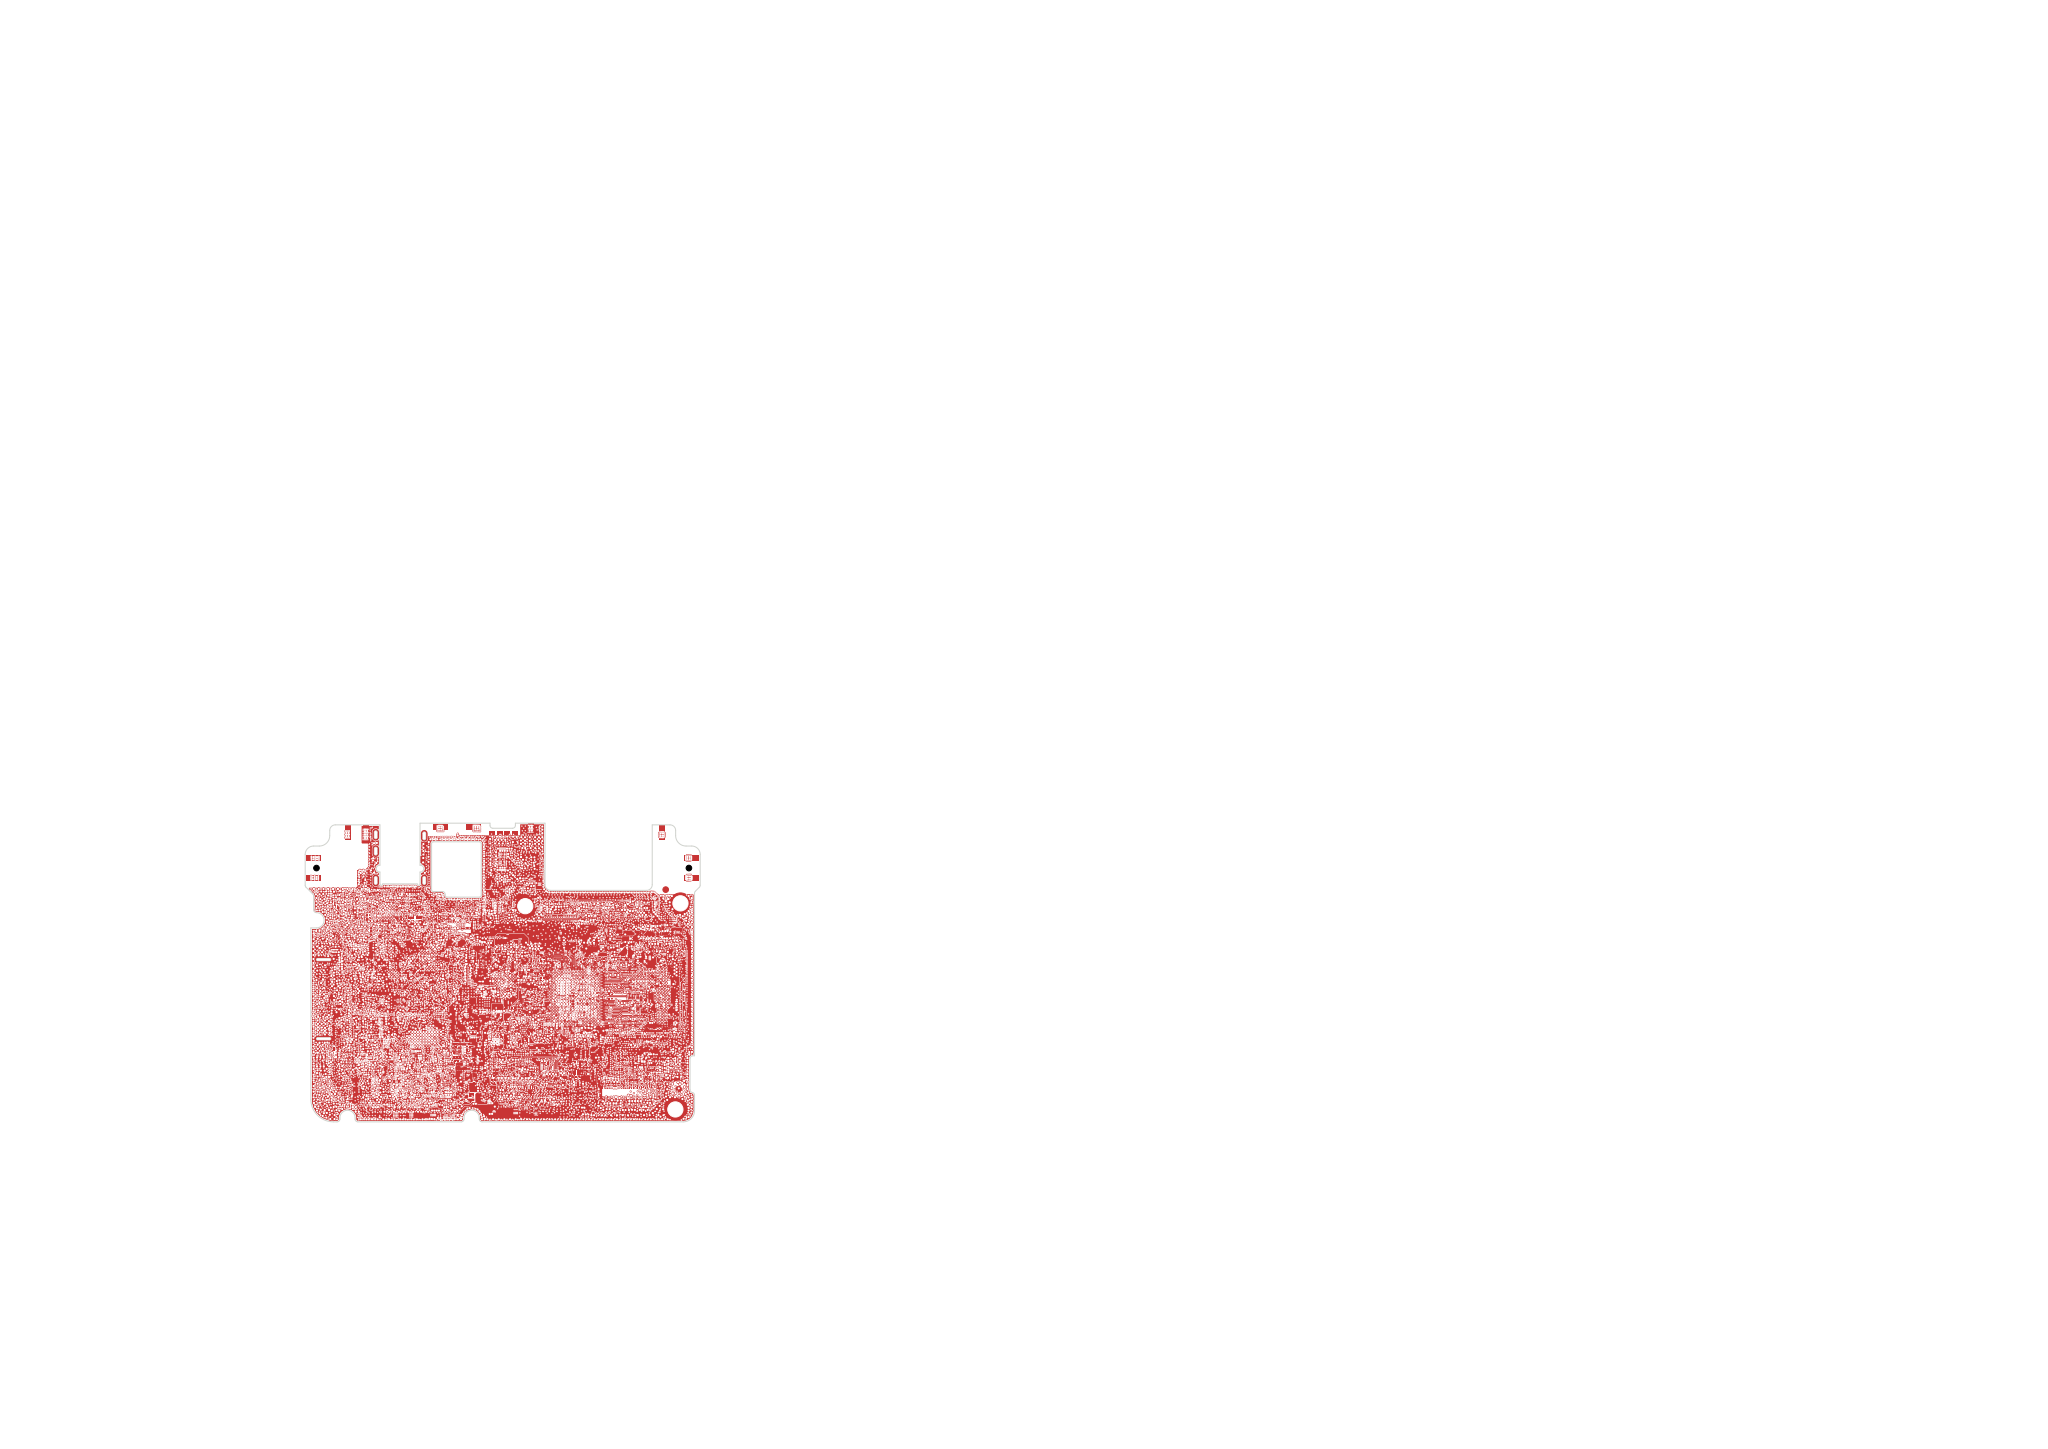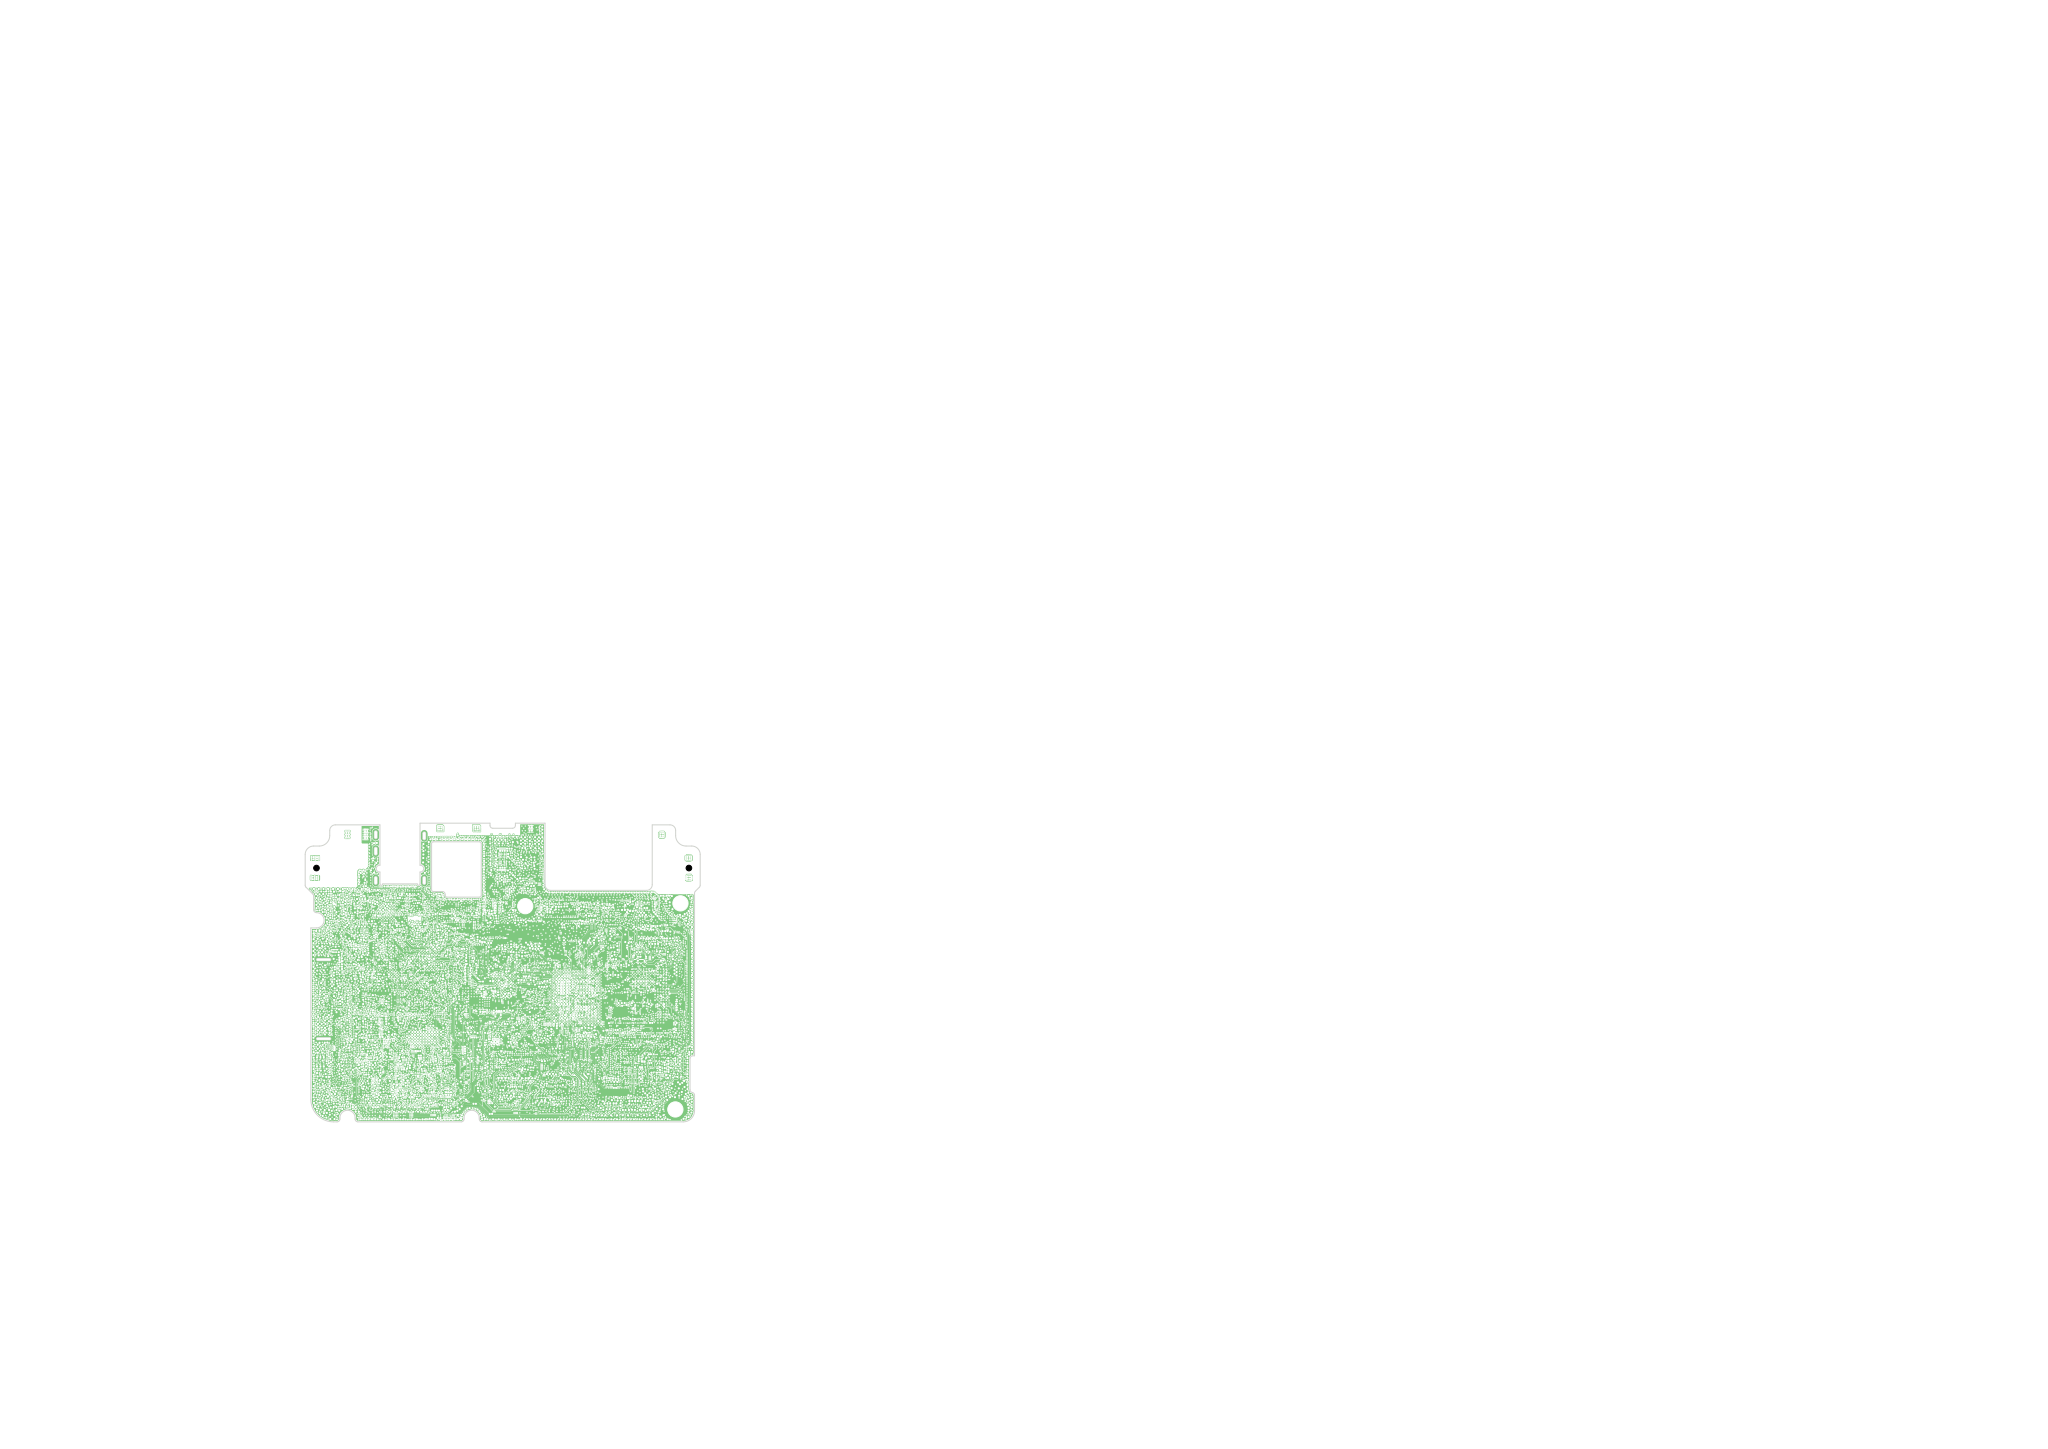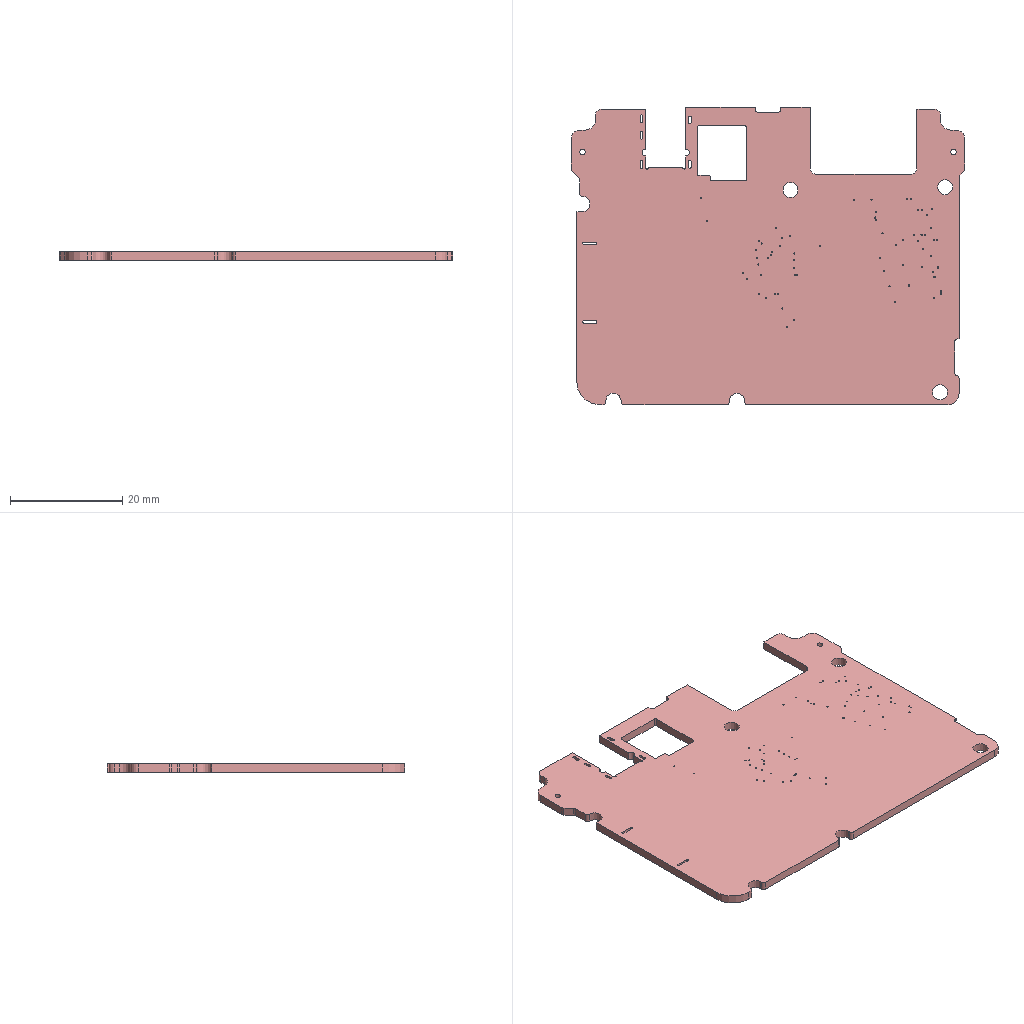Circuit board layout | KiCad | box 70 x 52.9 x 1.5 mm
Layer stack:
layer,type,thickness_mm,material,epsilon_r
F.Cu,copper (signal),,,
In1.Cu,copper (signal),,,
In2.Cu,copper (signal),,,
In3.Cu,copper (signal),,,
In4.Cu,copper (signal),,,
In5.Cu,copper (signal),,,
In6.Cu,copper (signal),,,
In7.Cu,copper (signal),,,
In8.Cu,copper (signal),,,
B.Cu,copper (signal),,,
# board thickness,1.6,,,
Part placement, first 811 of 1662 lines:
Ref,Val,Package,PosX,PosY,Rot,Side
B2102,,,26.012,28.75,-90,bottom
B2705,,,-11.025,38.45,180,bottom
C1101,,,9.938,26.938,-90,bottom
C1102,,,8.838,26.938,-90,bottom
C1103,,,12.137,24.312,0,bottom
C1104,,,12.137,23.712,0,bottom
C1105,,,11.387,26.3,-90,bottom
C1106,,,11.988,26.3,-90,bottom
C1107,,,12.137,24.913,0,bottom
C1108,,,12.588,25.988,-90,bottom
C1109,,,10.787,26.3,-90,bottom
C1111,,,9.338,19.5,180,bottom
C1122,,,8.2,21.7,0,bottom
C1123,,,9.338,18.4,180,bottom
C1124,,,8.2,20.6,0,bottom
C1125,,,9.938,23.712,0,bottom
C1126,,,9.938,23.113,0,bottom
C1127,,,9.938,22.512,0,bottom
C1128,,,11.037,24.913,180,bottom
C1129,,,11.037,23.712,180,bottom
C1130,,,11.037,23.113,180,bottom
C1131,,,6.237,17.288,0,bottom
C1132,,,8.537,17.288,180,bottom
C1133,,,11.6,20.712,180,bottom
C1134,,,9.938,24.913,0,bottom
C1135,,,11.037,19.95,180,bottom
C1136,,,10.5,21.312,0,bottom
C1137,,,10.5,20.712,0,bottom
C1138,,,11.6,21.312,180,bottom
C1139,,,11.037,24.312,180,bottom
C1140,,,11.037,22.512,180,bottom
C1170,,,9.938,24.312,0,bottom
C1171,,,14.463,29.062,0,bottom
C1172,,,14.463,30.163,0,bottom
C1173,,,12.387,22.863,90,bottom
C1174,,,15.8,25.137,0,bottom
C1175,,,14.7,25.137,180,bottom
C1176,,,13.225,23.15,-90,bottom
C1177,,,14.238,22.438,180,bottom
C1182,,,11.037,19.35,0,bottom
C1183,,,9.088,22.8,-90,bottom
C1201,,,11.04,18.75,180,bottom
C1202,,,15.537,20.212,0,bottom
C1203,,,13.225,24.25,90,bottom
C1204,,,9.65,20.962,90,bottom
C1205,,,13.338,19.2,0,bottom
C1211,,,18.2,22.562,-90,bottom
C1212,,,13.338,18.6,0,bottom
C1213,,,13.225,25.35,90,bottom
C1214,,,18.337,19.863,180,bottom
C1221,,,12.137,19.35,180,bottom
C1222,,,9.938,25.512,180,bottom
C1223,,,13.225,27.55,-90,bottom
C1224,,,13.225,26.45,90,bottom
C1225,,,15.537,18.413,0,bottom
C1231,,,11.037,18.15,180,bottom
C1232,,,11.6,21.913,0,bottom
C1241,,,10.588,17.3,90,bottom
C1242,,,17.038,17.562,180,bottom
C1243,,,15.537,19.012,180,bottom
C1244,,,14.438,19.012,0,bottom
C1245,,,14.438,18.413,0,bottom
C1246,,,14.438,20.4,180,bottom
C1247,,,14.438,19.8,180,bottom
C1248,,,15.537,19.613,180,bottom
C1249,,,14.338,17.562,0,bottom
C1251,,,15.55,25.988,-90,bottom
C1252,,,16.637,19.262,90,bottom
C1253,,,16.25,21.688,-90,bottom
C1254,,,18.337,18.762,180,bottom
C1255,,,15.15,23.938,180,bottom
C1256,,,15.15,23.337,180,bottom
C1257,,,13.338,19.913,0,bottom
C1258,,,13.338,20.512,0,bottom
C1259,,,13.338,21.113,0,bottom
C1260,,,14.488,21.587,-90,bottom
C1262,,,9.988,17.288,90,bottom
C1263,,,7.6,19.75,0,bottom
C1271,,,12.137,19.95,0,bottom
C1272,,,15.8,24.538,0,bottom
C1280,,,12.137,18.15,180,bottom
C1281,,,17.863,27.863,0,bottom
C1282,,,17.863,26.762,0,bottom
C1283,,,17.35,23.712,180,bottom
C1284,,,17.35,23.113,180,bottom
C1285,,,16.25,23.738,0,bottom
C1286,,,16.25,23.137,0,bottom
C1287,,,17.35,22.512,180,bottom
C1288,,,12.137,18.75,180,bottom
C1291,,,14.95,25.988,-90,bottom
C1501,,,2.15,28,-90,bottom
C1503,,,3.4,18.35,180,bottom
C1504,,,-2.05,27.7,180,bottom
C1507,,,0.1,29.65,180,bottom
C1508,,,1.025,20.2,0,bottom
C1509,,,-0.9375,18.637,0,bottom
C1519,,,1.587,18.337,180,bottom
C1525,,,2.45,30.3,-90,bottom
C1526,,,-0.25,31.1,-90,bottom
C1527,,,3.4,17.25,180,bottom
C1528,,,-1.85,28.5,180,bottom
C1529,,,-5.425,30.525,90,bottom
C1601,,,4.2,23.2,0,bottom
C1602,,,4.2,22.6,0,bottom
C1603,,,1.65,20.7,-90,bottom
C1604,,,4.05,26.95,0,bottom
C1605,,,3.9,30.3,0,bottom
C1606,,,3.9,31.4,0,bottom
C1607,,,4.188,25.125,0,bottom
C1612,,,4.812,25.875,0,bottom
C1613,,,-1.875,19.3,0,bottom
C1614,,,4.612,21.85,0,bottom
C1615,,,4.188,24.525,0,bottom
C1621,,,9.113,29.288,90,bottom
C1622,,,8.012,29.288,90,bottom
C1701,,,1.1,31.15,90,bottom
C1702,,,-4.1,27.25,180,bottom
C1703,,,0.95,27.95,90,bottom
C1704,,,-0.05,27.95,90,bottom
C1705,,,-1.55,29.5,90,bottom
C1706,,,-0.75,28.4,90,bottom
C1707,,,1.85,30.3,90,bottom
C1708,,,-3.9,25.85,180,bottom
C1709,,,-5.9,23,0,bottom
C1710,,,-4.1,28.05,180,bottom
C1711,,,11.162,29.988,90,bottom
C1712,,,1.05,29.55,90,bottom
C1713,,,0.1,30.25,180,bottom
C1714,,,-2.15,29.5,90,bottom
C1715,,,-0.95,29.5,90,bottom
C1716,,,-6.15,24,90,bottom
C1717,,,-5.15,26.45,180,bottom
C1718,,,-4.3,25,180,bottom
C1719,,,-3.9,26.55,0,bottom
C1720,,,-5.15,25.85,0,bottom
C1721,,,0.1,29.05,0,bottom
C1801,,,-4.15,24.125,90,bottom
C1802,,,-3.25,23.025,90,bottom
C1803,,,-1.09,20.575,-90,bottom
C1804,,,0.75,21.15,0,bottom
C1805,,,-4.9,23.85,90,bottom
C1807,,,-5.5,23.85,90,bottom
C1808,,,-0.75,19.35,180,bottom
C1809,,,-3.85,19.337,0,bottom
C1810,,,-1.475,16.837,180,bottom
C1811,,,-2.575,16.837,180,bottom
C1812,,,-3.4,23.9,90,bottom
C1828,,,-2.675,17.538,180,bottom
C1829,,,-5.1,22.15,180,bottom
C1834,,,-3.85,18.163,90,bottom
C1835,,,-4.525,17.175,90,bottom
C1901,,,24.5,21.85,-90,bottom
C1902,,,26.6,20.8,180,bottom
C1903,,,26.6,21.9,180,bottom
C1904,,,23.413,30,-90,bottom
C1905,,,23.212,17.3,90,bottom
C1906,,,23.1,18.663,-90,bottom
C1907,,,23.7,21.85,-90,bottom
C2001,,,22.2,22.1,-90,bottom
C2002,,,23.775,28.462,90,bottom
C2003,,,20.875,24.587,180,bottom
C2004,,,20.812,25.712,180,bottom
C2005,,,22.188,20.375,-90,bottom
C2006,,,20.7,29.65,90,bottom
C2007,,,19.413,26.812,90,bottom
C2008,,,19.812,28.012,180,bottom
C2009,,,22.538,19.525,0,bottom
C2010,,,30.375,20.775,0,bottom
C2011,,,28.175,21.275,-90,bottom
C2012,,,20.625,26.413,180,bottom
C2013,,,22.25,28.35,0,bottom
C2014,,,25.163,28.925,90,bottom
C2015,,,20.025,21.562,180,bottom
C2016,,,20.15,27.262,180,bottom
C2019,,,22.9,21.85,-90,bottom
C2020,,,22.788,20.375,-90,bottom
C2021,,,20.825,17.562,90,bottom
C2108,,,24.012,30,-90,bottom
C2109,,,24.613,30,90,bottom
C2110,,,25.212,30,90,bottom
C2111,,,28.01,28.348,0,bottom
C2118,,,26.812,28.75,-90,bottom
C2119,,,26.663,29.85,180,bottom
C2122,,,30.25,29.85,90,bottom
C2123,,,28.77,26.34,180,bottom
C2128,,,27.703,29.55,-90,bottom
C2129,,,25.812,30.1,90,bottom
C2130,,,28.378,30.65,180,bottom
C2131,,,26.075,31.25,180,bottom
C2132,,,26.075,31.85,180,bottom
C2133,,,26.925,31.6,90,bottom
C2134,,,28.375,31.85,180,bottom
C2135,,,27.525,31.6,90,bottom
C2201,,,28.45,22.125,180,bottom
C2202,,,29.05,22.875,0,bottom
C2203,,,28.2,23.775,180,bottom
C2204,,,31.3,25.25,-90,bottom
C2205,,,31.145,18.175,0,bottom
C2206,,,29.65,19.075,0,bottom
C2207,,,28.773,29.75,180,bottom
C2208,,,31.625,20.85,90,bottom
C2209,,,31.145,19.075,0,bottom
C2210,,,29.65,18.175,0,bottom
C2211,,,29,24.95,180,bottom
C2212,,,28.77,26.94,180,bottom
C2213,,,30.45,24.7,90,bottom
C2277,,,29.025,20.675,-90,bottom
C2707,,,-5.925,38.1,180,bottom
C2708,,,-12.475,38.45,-90,bottom
C2709,,,-6.675,37.5,0,bottom
C2710,,,-7.025,38.1,0,bottom
C2712,,,-9.325,37,180,bottom
C2718,,,2.875,41.95,90,bottom
C2730,,,6.25,42.8,180,bottom
C2731,,,4.225,42.8,0,bottom
C2732,,,5.025,40.6,0,bottom
C2755,,,-6.675,36.9,0,bottom
C3237,,,10.463,35.4,-90,bottom
C3238,,,9.863,35.4,-90,bottom
C3239,,,9.262,35.388,90,bottom
C3242,,,13.363,35.4,-90,bottom
C3243,,,9.662,39.612,90,bottom
C3244,,,14.887,39.625,-90,bottom
C3245,,,13.45,39.6,-90,bottom
C3246,,,14.05,39.6,-90,bottom
C3247,,,20.337,35.4,-90,bottom
C3248,,,19.738,35.4,-90,bottom
C3249,,,19.137,35.4,90,bottom
C3252,,,23.788,35.65,0,bottom
C3253,,,19.512,39.612,90,bottom
C3254,,,24.725,39.612,-90,bottom
C3255,,,24.125,39.612,-90,bottom
C3256,,,23.525,39.612,-90,bottom
C3351,,,0.7125,37.35,0,bottom
C3352,,,0,38.3,-90,bottom
C3702,,,11.588,14.8,0,bottom
C3713,,,6.388,14.2,180,bottom
C3717,,,14.599,9.125,90,bottom
C3718,,,10.75,10.05,90,bottom
C3719,,,9.55,10.05,90,bottom
C3800,,,-10.45,21.2,0,bottom
C3900,,,-15.975,25.85,-90,bottom
C3901,,,-16.15,28.75,0,bottom
C3902,,,-11.62,33.43,-90,bottom
C3903,,,-16.15,28.15,0,bottom
C3904,,,-11.7,34.675,0,bottom
C3905,,,-17.225,27.55,180,bottom
C3906,,,-10.375,34.3,90,bottom
C3907,,,-17,28.4,90,bottom
C3908,,,-10.97,34.3,90,bottom
C3909,,,-12,23.875,180,bottom
C3910,,,-15.125,25.575,180,bottom
C3911,,,-12.27,33.625,-90,bottom
C3912,,,-12.025,32.775,180,bottom
C3913,,,-12.85,23.975,90,bottom
C3914,,,-9.125,27.062,-90,bottom
C3915,,,-9.113,25.06,90,bottom
C3916,,,-9.75,29.82,-90,bottom
C3917,,,-9.515,34.935,180,bottom
C3918,,,-10,31.025,0,bottom
C3919,,,-9.1,30.975,90,bottom
C3920,,,-9.72,33.625,180,bottom
C3921,,,-10.885,33.195,90,bottom
C4001,,,-18.7,31.15,0,bottom
C4002,,,-10.5,32.075,-90,bottom
C4003,,,-19.8,31.15,0,bottom
C4004,,,-10.15,25.2,90,bottom
C4006,,,-18.6,30.55,0,bottom
C4007,,,-19.7,30.55,0,bottom
C4010,,,-19.7,29.95,0,bottom
C4011,,,-18.6,29.35,0,bottom
C4014,,,-17.275,34.15,180,bottom
C4015,,,-18.7,33.538,0,bottom
C4019,,,-18.6,29.95,0,bottom
C4020,,,-18.2,28.475,90,bottom
C4021,,,-18.7,32.95,0,bottom
C4022,,,-19.8,32.95,0,bottom
C4024,,,-19.8,32.35,0,bottom
C4026,,,-17.6,32.35,0,bottom
C4028,,,-19.8,31.75,0,bottom
C4029,,,-17.6,31.75,0,bottom
C4031,,,-15.425,33.175,-90,bottom
C4034,,,-14.825,33.175,-90,bottom
C4043,,,-14.225,33.775,-90,bottom
C4045,,,-15.075,34,0,bottom
C4046,,,-13.625,33.775,-90,bottom
C4047,,,-14.225,34.875,-90,bottom
C4048,,,-13.025,33.775,-90,bottom
C4049,,,-13.025,34.875,-90,bottom
C4050,,,-16.212,17.887,90,bottom
C4059,,,-15,17.887,90,bottom
C4062,,,-11.387,25.038,0,bottom
C4070,,,-17.6,17.887,90,bottom
C4071,,,-9.65,32.237,180,bottom
C4072,,,-12,24.475,0,bottom
C4073,,,-10.035,32.945,180,bottom
C4101,,,-12.75,11.725,0,bottom
C4102,,,-9.5,11.95,180,bottom
C4103,,,-18.575,15.675,0,bottom
C4104,,,-17.725,15.325,90,bottom
C4105,,,-12.562,17.887,-90,bottom
C4106,,,-11.463,17.738,180,bottom
C4107,,,-17.975,16.438,180,bottom
C4108,,,-15.61,17.885,90,bottom
C4110,,,-16.812,17.887,90,bottom
C4112,,,-9.537,17.038,0,bottom
C4114,,,-10.113,17.637,0,bottom
C4116,,,-9.537,16.4,0,bottom
C4117,,,-13.762,17.887,-90,bottom
C4118,,,-14.363,17.887,-90,bottom
C4119,,,-11.925,9.925,0,bottom
C4201,,,-27.45,14.3,0,bottom
C4301,,,-25.887,33.688,180,bottom
C4302,,,-22.975,31.55,180,bottom
C4304,,,-19.95,9.425,0,bottom
C4305,,,-22.125,18.288,0,bottom
C4306,,,-22.125,17.688,0,bottom
C4307,,,-24.9,18.2,0,bottom
C4308,,,-24.075,15.975,90,bottom
C4309,,,-20.9,32.45,180,bottom
C4310,,,-23.375,33.413,0,bottom
C4311,,,-19.325,17.188,0,bottom
C4312,,,-20.075,15.137,90,bottom
C4313,,,-20.275,34.938,180,bottom
C4314,,,-22.425,34.875,90,bottom
C4401,,,-18.9,4.525,180,bottom
C4402,,,-11.35,6.55,-90,bottom
C4403,,,-16.562,5.05,-90,bottom
C4405,,,-13.625,6.575,-90,bottom
C4406,,,-20.275,34.337,180,bottom
C4407,,,-18.125,34.388,-90,bottom
C4501,,,-24.775,7.175,180,bottom
C4502,,,-20.72,4.575,-90,bottom
C4503,,,-28.225,10.3,90,bottom
C4504,,,-28.875,11.2,180,bottom
C4505,,,-25.375,5.2,180,bottom
C4506,,,-25.375,8,180,bottom
C4507,,,-29.225,7.425,180,bottom
C4508,,,-29.525,12.725,90,bottom
C4601,,,-29.1,33.175,180,bottom
C4602,,,-23.4,26.775,-90,bottom
C4603,,,-22.975,30.95,180,bottom
C4604,,,-24.73,28.81,0,bottom
C4605,,,-25.65,25.2,-90,bottom
C4606,,,-23.825,28.975,-90,bottom
C4607,,,-11.975,20.125,180,bottom
C4609,,,-25.45,22.5,90,bottom
C4610,,,-24.45,20.95,180,bottom
C4611,,,-19.375,22.7,180,bottom
C4612,,,-19.7,20.7,-90,bottom
C4613,,,-19.7,21.8,-90,bottom
C4614,,,-24.9,24.788,90,bottom
C4616,,,-24.05,25.525,180,bottom
C4617,,,-18.825,20.875,180,bottom
C4701,,,-16.875,26.375,-90,bottom
C4702,,,-19.125,23.775,0,bottom
C4703,,,-17.475,26.375,-90,bottom
C4704,,,-19.125,24.375,0,bottom
C4706,,,-21.45,25.35,0,bottom
C4708,,,-14.775,21.875,90,bottom
C4709,,,-14.175,21.875,90,bottom
C4710,,,-16.275,24.675,-90,bottom
C4711,,,-16.875,24.675,-90,bottom
C4712,,,-16.875,23.575,90,bottom
C4713,,,-16.275,23.575,90,bottom
C4801,,,-28.45,21.05,-90,bottom
C4802,,,-28.2,21.95,180,bottom
C4901,,,1.85,41.525,180,bottom
C4902,,,0.775,39.7,90,bottom
C5105,,,-15.125,20.2,180,bottom
C5601,,,-29.25,41.1,180,bottom
C5602,,,-29.288,37.288,180,bottom
C5617,,,28.488,38.25,180,bottom
C5620,,,-25.127,37.913,0,bottom
C5621,,,-22.913,39.062,180,bottom
C5622,,,-24.702,40.263,180,bottom
C5623,,,-25.802,39.062,180,bottom
C5624,,,-25.802,40.263,0,bottom
C5625,,,-24.027,37.913,180,bottom
C5626,,,-23.175,38.163,-90,bottom
C5628,,,-21.975,38.163,90,bottom
C5629,,,-23.602,40.263,0,bottom
C5630,,,-22.502,40.263,180,bottom
C5631,,,-18.587,37.962,180,bottom
C5801,,,-3.962,9.703,90,bottom
C5803,,,-0.125,13.512,-90,bottom
C5804,,,-4.425,5.75,-90,bottom
C5805,,,-3.525,5.725,90,bottom
C5806,,,-1.55,13.512,-90,bottom
C5807,,,0.85,13.512,-90,bottom
C5808,,,-0.8375,13.262,-90,bottom
C5809,,,-5.675,7.375,0,bottom
C5810,,,-5.675,8.988,0,bottom
C5811,,,-3.05,13.512,-90,bottom
C5812,,,-4.35,7.25,-90,bottom
C5813,,,0.54,7.835,90,bottom
C5814,,,-5.675,8.188,0,bottom
C5815,,,-5.412,10.488,0,bottom
C5816,,,-5.675,9.787,180,bottom
C5817,,,-2.388,13.25,-90,bottom
C5818,,,0.29,5.04,180,bottom
C5819,,,-2.505,5.985,90,bottom
C5820,,,0.29,5.64,180,bottom
C5821,,,1.145,5.39,90,bottom
C5822,,,0.29,4.44,0,bottom
C5823,,,-1.91,6.84,180,bottom
C5824,,,-1.42,4.54,180,bottom
C5825,,,-0.565,4.89,-90,bottom
C5826,,,-1.42,3.94,180,bottom
C5827,,,-1.42,5.14,180,bottom
C5828,,,-3.638,11.012,90,bottom
C5829,,,-5.588,11.25,0,bottom
C5830,,,0.29,6.84,0,bottom
C5831,,,-0.81,6.84,180,bottom
C5832,,,1.265,11.06,90,bottom
CR2201,,,30.45,25.95,0,bottom
D1801,,,-3.1,18.387,180,bottom
D2701,,,-10.175,37.462,90,bottom
D2705,,,-5.812,38.7,0,bottom
D2712,,,2.837,42.8,180,bottom
D2714,,,5.037,42.8,180,bottom
D3201,,,0,44.612,-90,bottom
D3202,,,0,48.388,90,bottom
D3502,,,-32.3,10.635,90,bottom
D3505,,,-31.7,10.635,90,bottom
D3506,,,-32.9,10.635,90,bottom
D3701,,,15.562,9.375,0,bottom
D3702,,,8,10.338,90,bottom
D3703,,,9.887,14.062,-90,bottom
D3704,,,11.35,10.162,90,bottom
D3705,,,8.95,10.338,90,bottom
D3706,,,11.05,14.1,180,bottom
D3707,,,12.688,14.662,-90,bottom
D3708,,,9.287,14.062,-90,bottom
D3712,,,13.25,15.025,180,bottom
D3713,,,8.488,9.375,0,bottom
D3714,,,6.997,9.375,180,bottom
D3715,,,10.15,10.338,90,bottom
D3716,,,12.8,10.338,90,bottom
D3717,,,12.2,10.338,90,bottom
D3719,,,13.4,10.338,90,bottom
D3720,,,14,10.338,90,bottom
D3721,,,15.2,10.338,90,bottom
D3722,,,12.162,9.2,180,bottom
D3723,,,7.487,14.062,-90,bottom
D3724,,,8.088,14.062,-90,bottom
D3725,,,11.637,9.2,0,bottom
D3726,,,13.287,14.062,-90,bottom
D3727,,,11.975,14.1,180,bottom
D3728,,,7.4,10.338,90,bottom
D3729,,,8.688,14.062,-90,bottom
D3730,,,13.887,14.062,-90,bottom
D3731,,,9.213,9.2,180,bottom
D3732,,,15.089,14.063,-90,bottom
D3733,,,10.488,14.062,-90,bottom
D3734,,,14.038,9.375,0,bottom
D3738,,,14.488,14.063,-90,bottom
D3739,,,14.6,10.338,90,bottom
FL4201,,,-21.975,11.925,90,bottom
FL4202,,,-24.8,11.35,180,bottom
FL4203,,,-25.843,8.865,0,bottom
FL4301,,,-19.625,14.2,90,bottom
FL4302,,,-19.413,40.263,90,bottom
FL4303,,,-25.038,33.188,180,bottom
FL4304,,,-18.05,10.915,90,bottom
FL4305,,,-19.025,8.775,180,bottom
FL4401,,,-18.85,6.225,180,bottom
FL4402,,,-12.1,9.075,180,bottom
FL4403,,,-16.488,6.95,180,bottom
FL4404,,,-14.275,9.075,180,bottom
FL4501,,,-28.325,5.825,-90,bottom
FL4601,,,-25.788,32.062,180,bottom
FL4602,,,-23.25,29.2,180,bottom
FL4603,,,-21.525,31.4,180,bottom
FL4604,,,-21.825,30.288,180,bottom
FL4605,,,-11.775,21.35,-90,bottom
FL4607,,,-24.775,21.65,-90,bottom
FL4608,,,-18.5,22.075,180,bottom
FL4609,,,-24.25,23.875,180,bottom
FL4611,,,-22.75,24.95,-90,bottom
FL4612,,,-17.375,20.675,180,bottom
FL4701,,,-25.035,34.663,180,bottom
FL4702,,,-14.225,20.575,180,bottom
FL5605,,,-19.538,37.888,0,bottom
FL5702,,,-9.6,23.613,0,bottom
J2705,,,4.117,46.83,90,bottom
J3202,,,14.863,38.675,0,bottom
J3203,,,24.75,38.675,0,bottom
J3501,,,-31.62,8.4,90,bottom
J3603,,,-10.1,3.237,0,bottom
J3701,,,6.8,13.4,180,bottom
J3702,,,20.88,13.15,90,bottom
J4503,,,-29.5,16.238,-90,bottom
J4601,,,-29.5,32.275,90,bottom
J4802,,,-29.3,25.225,0,bottom
J4902,,,-4.55,51.9,0,bottom
J4903,,,-11.25,51.9,180,bottom
J4905,,,32.95,43.2,180,bottom
J4909,,,4.75,51.9,180,bottom
J4911,,,-2.3,38.675,180,bottom
J5601,,,-32.95,46.7,0,bottom
J5602,,,-29.512,38.04,-90,bottom
J5603,,,-24.5,50.837,-90,bottom
J5604,,,-32.95,43.2,0,bottom
J5610,,,28.25,50.837,-90,bottom
J5611,,,-27.5,50.85,-90,bottom
J5612,,,32.95,46.7,180,bottom
J5613,,,-14.9,40.05,90,bottom
J5615,,,29.5,35.675,180,bottom
J5616,,,-6,35.837,180,bottom
J5801,,,7.5,2.25,90,bottom
J5802,,,4.5,2.25,90,bottom
L1601,,,5.34,23.25,180,bottom
L1602,,,6.05,21.85,90,bottom
L1603,,,2.65,19.9,180,bottom
L1604,,,3.6,27.75,-90,bottom
L1605,,,5.6,27.155,-90,bottom
L1606,,,6.188,24.75,-90,bottom
L1801,,,-3.45,20.75,180,bottom
L1901,,,25.1,19.25,180,bottom
L2001,,,22.1,29.15,-90,bottom
L2002,,,20.7,20.512,90,bottom
L2003,,,20.9,23.012,0,bottom
L2004,,,19.7,25.012,0,bottom
L2005,,,19.863,29.413,0,bottom
L2201,,,30.55,27.05,-90,bottom
L2202,,,30.775,23.425,90,bottom
L2701,,,-8.475,37.35,90,bottom
L2706,,,-8.725,38.45,180,bottom
L4001,,,-17.6,31.15,0,bottom
L4003,,,-16.5,31.15,0,bottom
L4006,,,-17.5,30.55,0,bottom
L4007,,,-16.4,30.55,0,bottom
L4010,,,-17.5,29.95,0,bottom
L4011,,,-16.4,29.95,0,bottom
L4012,,,-17.6,29.025,90,bottom
L4016,,,-17.6,32.95,0,bottom
L4018,,,-16.4,29.35,0,bottom
L4019,,,-17.6,33.538,0,bottom
L4020,,,-16.5,33.538,0,bottom
L4022,,,-16.5,32.95,0,bottom
L4024,,,-18.7,32.35,0,bottom
L4026,,,-16.5,32.35,0,bottom
L4028,,,-18.7,31.75,0,bottom
L4029,,,-16.5,31.75,0,bottom
L4034,,,-15.075,32.325,0,bottom
L4045,,,-14.225,32.675,-90,bottom
L4055,,,-13.625,32.675,-90,bottom
L4057,,,-13.025,32.675,-90,bottom
L4061,,,-13,25.625,180,bottom
L4062,,,-12.488,25.038,180,bottom
L4071,,,-18.2,17.887,-90,bottom
L4101,,,-11.65,11.725,180,bottom
L4102,,,-9.5,12.55,180,bottom
L4109,,,-10.55,11.35,180,bottom
L4110,,,-10.2,10.5,-90,bottom
L4111,,,-9.775,14.075,90,bottom
L4112,,,-9.175,14.075,90,bottom
L4113,,,-9.525,13.225,180,bottom
L4201,,,-19.425,15.425,90,bottom
L4202,,,-22.95,13.45,-90,bottom
L4203,,,-22.675,10.025,90,bottom
L4204,,,-21.475,10.025,-90,bottom
L4205,,,-24.675,13.425,-90,bottom
L4206,,,-27.75,13.65,180,bottom
L4207,,,-27.4,12.8,-90,bottom
L4208,,,-23.325,12,180,bottom
L4209,,,-23.325,12.6,180,bottom
L4210,,,-23.525,9.7,180,bottom
L4211,,,-21.9,9.1,180,bottom
L4212,,,-23.325,14.925,180,bottom
L4213,,,-25.25,14.3,0,bottom
L4214,,,-25.3,15.15,-90,bottom
L4215,,,-25.125,8.85,90,bottom
L4216,,,-26.525,11.175,180,bottom
L4217,,,-26.525,10.575,180,bottom
L4218,,,-24.275,9.1,0,bottom
L4301,,,-20,11.375,180,bottom
L4302,,,-18.925,14.225,90,bottom
L4303,,,-17.725,14.225,-90,bottom
L4304,,,-18.363,39.438,-90,bottom
L4305,,,-20.712,40.263,0,bottom
L4306,,,-18.587,38.587,180,bottom
L4307,,,-18.113,40.288,180,bottom
L4308,,,-20.712,39.663,0,bottom
L4309,,,-21.65,40.013,90,bottom
L4310,,,-18.925,13.125,-90,bottom
L4311,,,-17.725,13.125,90,bottom
L4312,,,-20,11.975,180,bottom
L4313,,,-22.35,13.455,90,bottom
L4314,,,-25.887,33.087,0,bottom
L4315,,,-23.225,32.562,-90,bottom
L4316,,,-22.6,14.305,0,bottom
L4317,,,-17.15,9.525,180,bottom
L4318,,,-19.95,10.625,0,bottom
L4319,,,-24.675,15.75,90,bottom
L4320,,,-23.225,16.5,0,bottom
L4321,,,-17.025,8.575,90,bottom
L4322,,,-23.575,17.35,90,bottom
L4323,,,-16.625,11.475,90,bottom
L4324,,,-19.55,18.137,-90,bottom
L4325,,,-17.95,7.125,180,bottom
L4326,,,-19.9,7.475,-90,bottom
L4327,,,-20.675,17.938,-90,bottom
L4330,,,-22.425,33.775,-90,bottom
L4331,,,-22.163,33.513,180,bottom
L4332,,,-20.9,33.05,0,bottom
L4333,,,-20.9,33.65,180,bottom
L4344,,,-18.68,12.215,0,bottom
L4345,,,-18.68,11.615,0,bottom
L4346,,,-17.825,11.965,90,bottom
L4347,,,-17.225,11.475,90,bottom
L4401,,,-19.75,4.575,-90,bottom
L4402,,,-16.025,11.475,-90,bottom
L4403,,,-13.45,10.525,0,bottom
L4404,,,-15.775,10.625,180,bottom
L4405,,,-15.425,11.475,90,bottom
L4406,,,-13.025,9.925,0,bottom
L4407,,,-13.45,11.125,180,bottom
L4408,,,-13.625,34.875,-90,bottom
L4409,,,-17.8,4.525,180,bottom
L4410,,,-11.1,5.7,180,bottom
L4411,,,-11.1,7.4,180,bottom
L4412,,,-15.475,9.062,-90,bottom
L4413,,,-14.3,10.875,-90,bottom
L4414,,,-15.225,8.213,180,bottom
L4415,,,-15.225,9.912,180,bottom
L4416,,,-14.125,9.925,0,bottom
L4417,,,-14.55,11.725,0,bottom
L4418,,,-16.312,4.2,180,bottom
L4419,,,-15.713,5.3,180,bottom
L4420,,,-13.363,5.725,180,bottom
L4421,,,-13.365,7.425,180,bottom
L4422,,,-17.275,34.75,0,bottom
L4423,,,-16.175,34.75,180,bottom
L4424,,,-15.075,35.125,180,bottom
L4425,,,-15.075,34.562,0,bottom
L4501,,,-24.525,8.1,90,bottom
L4502,,,-25.65,7.15,-90,bottom
L4503,,,-24.525,4.95,90,bottom
L4504,,,-25.65,6.05,-90,bottom
L4505,,,-29.225,6.825,0,bottom
L4506,,,-29.225,8.025,180,bottom
L4507,,,-29.275,11.875,180,bottom
L4508,,,-29.275,13.575,180,bottom
L4509,,,-20.47,5.425,180,bottom
L4510,,,-20.47,6.025,180,bottom
L4601,,,-30.2,33.175,0,bottom
L4602,,,-23.4,27.875,-90,bottom
L4603,,,-22.55,27.55,0,bottom
L4604,,,-28.25,33.425,-90,bottom
L4605,,,-24.73,29.41,0,bottom
L4607,,,-22.125,31.212,-90,bottom
L4608,,,-19.4,28.475,90,bottom
L4609,,,-22.7,30.35,0,bottom
L4610,,,-21.7,28.375,-90,bottom
L4611,,,-21.1,28.375,-90,bottom
L4612,,,-22.55,24.35,0,bottom
L4613,,,-11.975,20.725,0,bottom
L4614,,,-11.6,23.025,-90,bottom
L4617,,,-25.7,21.65,0,bottom
L4620,,,-25.3,20.7,90,bottom
L4621,,,-23.6,20.7,90,bottom
L4622,,,-19.1,21.8,90,bottom
L4623,,,-16.825,21.85,180,bottom
L4624,,,-24.9,23.688,90,bottom
L4625,,,-22.55,23.75,0,bottom
L4626,,,-22.95,21.725,90,bottom
L4628,,,-22.55,26.35,0,bottom
L4629,,,-24.05,24.925,0,bottom
L4630,,,-17.975,20.625,90,bottom
L4631,,,-15.975,20.45,90,bottom
L4632,,,-22.55,23.15,180,bottom
L4633,,,-20.35,23.3,180,bottom
L4634,,,-25.83,29.41,180,bottom
L4701,,,-21.45,25.95,0,bottom
L4702,,,-23.288,35.125,0,bottom
L4703,,,-23.025,34.275,-90,bottom
L4704,,,-25.887,34.925,0,bottom
L4705,,,-25.887,34.325,180,bottom
L4707,,,-15.375,21.875,-90,bottom
L4708,,,-13.575,21.875,-90,bottom
L4709,,,-11.15,24.125,-90,bottom
L4710,,,-11,23.025,90,bottom
L4713,,,-22.55,26.95,0,bottom
L4715,,,-20,28.975,90,bottom
L4716,,,-22.55,28.15,0,bottom
L4717,,,-21.45,23.55,0,bottom
L4801,,,-30.8,23.125,90,bottom
L4802,,,-29.62,20.06,0,bottom
L4804,,,-29.35,22.275,180,bottom
L4805,,,-29,23.125,90,bottom
L4806,,,-30.72,19.46,0,bottom
L4807,,,-30.975,21.05,-90,bottom
L4808,,,-30.45,22.275,0,bottom
L4809,,,1.85,40.325,180,bottom
L4810,,,1.375,39.475,90,bottom
L5102,,,-12.825,20.375,90,bottom
L5103,,,-15.125,20.8,0,bottom
L5601,,,-29.25,42.8,180,bottom
L5602,,,-28.938,36.438,-90,bottom
L5605,,,28.488,39.95,180,bottom
L5606,,,-25.802,39.663,180,bottom
L5607,,,-22.502,39.663,0,bottom
L5608,,,-17.738,38.2,90,bottom
L5801,,,-5.925,4.425,180,bottom
L5802,,,-3.36,7.22,90,bottom
L5803,,,-1.655,7.815,180,bottom
M3701,,,31.415,5.76,0,bottom
M3702,,,32.485,35.25,0,bottom
M3703,,,-30.925,2.15,0,bottom
R0502,,,10.113,15.925,180,bottom
R1101,,,22.25,17.913,-90,bottom
R1201,,,16.9,25.212,-90,bottom
R1202,,,12.037,17.3,180,bottom
R1208,,,12.525,27.65,-90,bottom
R1502,,,-0.9375,18.038,0,bottom
R1503,,,-0.9375,17.438,0,bottom
R1505,,,0.35,31.1,-90,bottom
R1509,,,0.5625,18.587,90,bottom
R1510,,,1.587,17.738,180,bottom
R1517,,,1.663,19.212,90,bottom
R1518,,,-0.85,31.1,90,bottom
R1520,,,0.8125,19.438,180,bottom
R1523,,,0.4875,17.738,180,bottom
R1524,,,1.587,17.137,0,bottom
R1603,,,8.838,24.637,-90,bottom
R1604,,,6.2,29.61,180,bottom
R1605,,,6.713,18.65,180,bottom
R1701,,,8.075,31.425,180,bottom
R1803,,,-5.2,27.3,-90,bottom
R1804,,,-5.9,27.55,90,bottom
R1866,,,-6,26.2,90,bottom
R1867,,,-6,25.1,-90,bottom
R1868,,,-5.95,21.05,-90,bottom
R1874,,,-3.675,16.837,180,bottom
R1901,,,23.7,20.25,-90,bottom
R1903,,,22.562,31.85,180,bottom
R2028,,,18.25,21.212,0,bottom
R2031,,,19.95,31,0,bottom
R2032,,,19.337,17.562,0,bottom
R2101,,,28.375,31.25,0,bottom
R2120,,,23.512,31.35,-90,bottom
R2121,,,24.312,31.35,-90,bottom
R2122,,,25.113,31.35,-90,bottom
R2201,,,31.45,29.85,-90,bottom
R2202,,,30.85,29.85,-90,bottom
R2703,,,-10.775,37.35,-90,bottom
R2704,,,-11.625,37,0,bottom
R2705,,,-12.475,37.35,90,bottom
R2706,,,-11.625,37.6,180,bottom
R2707,,,-5.825,37.25,90,bottom
R2709,,,-7.025,38.7,180,bottom
R2730,,,5.175,41.7,90,bottom
R2731,,,4.375,41.7,90,bottom
R2735,,,3.575,41.7,90,bottom
R2740,,,-9.325,37.6,180,bottom
R2741,,,-7.875,37.35,-90,bottom
R3201,,,10.213,29.288,90,bottom
R3207,,,15.738,39.375,0,bottom
R3209,,,25.575,39.362,0,bottom
R3302,,,0.85,38.05,0,bottom
R3501,,,-32.9,11.5,-90,bottom
R3502,,,-32.3,11.5,-90,bottom
R3503,,,-31.7,11.5,-90,bottom
R3504,,,-25.137,43.825,180,bottom
R3505,,,-25.137,43.225,180,bottom
R3506,,,-24.288,43.475,90,bottom
R3701,,,10.425,9.2,0,bottom
R3800,,,-10.7,20.35,-90,bottom
R3801,,,-10.325,26.05,0,bottom
R3802,,,-10.325,26.65,0,bottom
R3900,,,-9.125,25.962,90,bottom
R3901,,,-9.41,31.64,180,bottom
R4000,,,-16.175,34.15,0,bottom
R4101,,,-11.988,11.125,180,bottom
R4102,,,-13.162,17.887,-90,bottom
R4103,,,-18.575,15.075,0,bottom
R4104,,,-17.975,17.038,180,bottom
R4109,,,-9.35,10.25,0,bottom
R4110,,,-10.8,10.5,-90,bottom
R4112,,,-11.988,10.525,180,bottom
R4201,,,-19.175,16.275,180,bottom
R4202,,,-23.8,13.4,0,bottom
R4203,,,-22.075,10.025,-90,bottom
R4204,,,-28,12.8,-90,bottom
R4205,,,-24.425,12.575,0,bottom
R4206,,,-25.575,11.525,90,bottom
R4207,,,-23,9.1,0,bottom
R4208,,,-24.15,14.3,180,bottom
R4209,,,-25.9,15.15,-90,bottom
R4210,,,-26.525,11.775,180,bottom
R4211,,,-27.375,10.85,-90,bottom
R4212,,,-26.35,14.3,0,bottom
R4213,,,-24.775,9.7,0,bottom
R4301,,,-20.875,10.525,-90,bottom
R4302,,,-18.325,14.225,90,bottom
R4303,,,-18.325,13.125,-90,bottom
R4304,,,-20.85,11.625,-90,bottom
R4305,,,-17.23,10.375,90,bottom
R4306,,,-19.95,10.025,0,bottom
R4307,,,-25.91,16.26,-90,bottom
R4308,,,-25.91,17.36,90,bottom
R4309,,,-25.91,17.88,90,bottom
R4311,,,-25.65,16,180,bottom
R4312,,,-23.8,18.2,180,bottom
R4313,,,-23.225,15.9,180,bottom
R4314,,,-22.975,17.35,90,bottom
R4315,,,-16.625,10.375,-90,bottom
R4316,,,-18.95,18.137,-90,bottom
Pad and via stacks:
via_type,start_layer,end_layer,diameter_mm,drill_mm,count
through,F.Cu,B.Cu,0.2,0.075,19915
through,F.Cu,B.Cu,0.4,0.2,2592
Design rules, without the lines most boards share:
# KiCad design rules of  (unit mm). No .kicad_pro was delivered with this board (it is a KiCad conversion), so the rules are the board's own setup values and the widths actually used on the board.
pad_to_mask_clearance = 0
allow_soldermask_bridges_in_footprints = no
capping = no
filling = no
# track widths used (mm): count
track_width 0.05 count=10171
track_width 0.0501 count=39
track_width 0.055 count=892
track_width 0.057 count=190
track_width 0.06 count=7392
track_width 0.061 count=2
track_width 0.0635 count=78
track_width 0.064 count=50
track_width 0.065 count=92
track_width 0.0664 count=12
track_width 0.07 count=30
track_width 0.073 count=1011
track_width 0.075 count=690
track_width 0.08 count=8
track_width 0.1 count=2271
track_width 0.11 count=3
track_width 0.12 count=432
track_width 0.13 count=9
track_width 0.14 count=6
track_width 0.15 count=2972
track_width 0.17 count=1
track_width 0.18 count=34
track_width 0.185 count=1
track_width 0.19 count=133
track_width 0.195 count=1
track_width 0.1984 count=5
track_width 0.2 count=6372
track_width 0.2025 count=56
track_width 0.22 count=15
track_width 0.227 count=2
track_width 0.228 count=185
track_width 0.25 count=534
track_width 0.3 count=337
track_width 0.35 count=63
track_width 0.4 count=78
track_width 0.45 count=5
track_width 0.5 count=147
track_width 0.55 count=4
track_width 0.6 count=5
track_width 0.7 count=7
track_width 0.8 count=25
track_width 0.9 count=14
track_width 1 count=20
# copper zones (pour): pad connection, clearance mm, minimum width mm, count
Classes set for this board:
# KiCad net classes of . No .kicad_pro was delivered with this board, so every net is in the KiCad Default class; nets on the board: 0
{"name": "Default", "nets": 0}